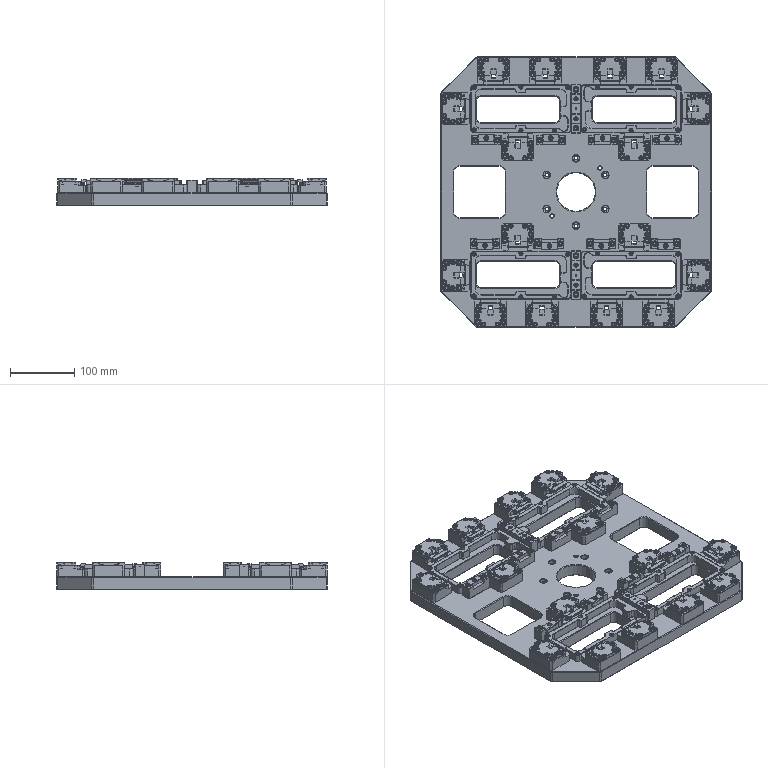Part | SolidWorks | features InContextFeatHolder 7, Attribute 1, LocalCirPattern 1, ReferencePattern 1 | 363 solids | 14362 faces | volume 3131018 mm3 | plane 5952 | cylinder 3806 | cone 3276 | torus 1104 | sphere 224 | commonest cylinder face diameters 4 x672 3 x548 2 x336 6.5 x264 5.5 x188 4.5 x176